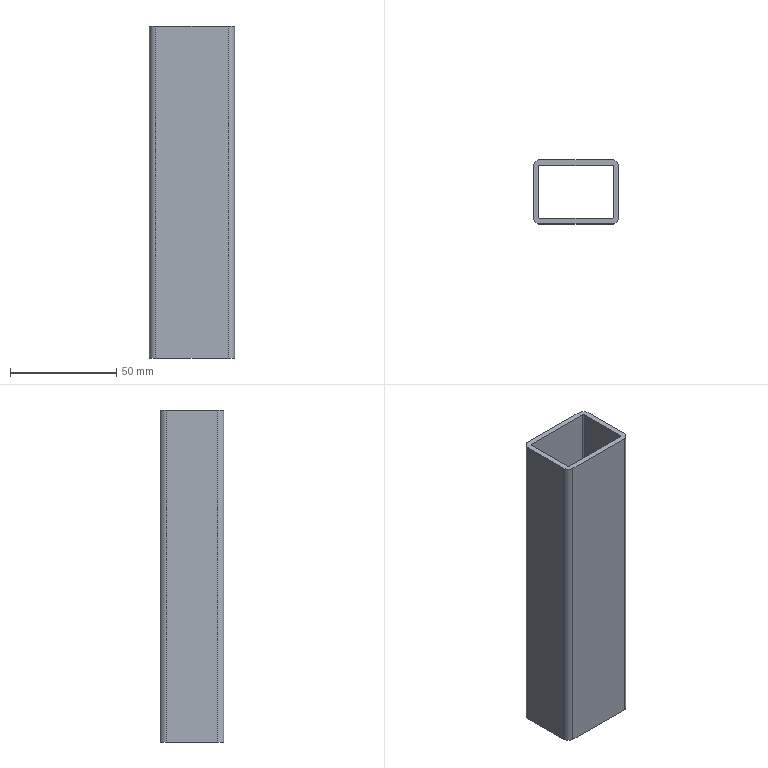Part | SolidWorks | features BaseBody 1 | 1 solid | 18 faces | box 40 x 30 x 156 mm | volume 49528 mm3 | plane 10 | cylinder 8 | commonest cylinder face diameters 1 x4 6 x4
STEP:
#1=CARTESIAN_POINT('',(17.,12.5,-78.));
#2=VERTEX_POINT('',#1);
#3=CARTESIAN_POINT('',(-17.,12.5,-78.));
#4=VERTEX_POINT('',#3);
#5=CARTESIAN_POINT('',(-17.,12.5,-78.));
#6=DIRECTION('',(-1.,0.,0.));
#7=VECTOR('',#6,1000.);
#8=LINE('',#5,#7);
#9=EDGE_CURVE('',#2,#4,#8,.T.);
#10=ORIENTED_EDGE('',*,*,#9,.F.);
#11=CARTESIAN_POINT('',(17.,12.5,78.));
#12=VERTEX_POINT('',#11);
#13=CARTESIAN_POINT('',(17.,12.5,78.));
#14=DIRECTION('',(0.,0.,-1.));
#15=VECTOR('',#14,1000.);
#16=LINE('',#13,#15);
#17=EDGE_CURVE('',#12,#2,#16,.T.);
#18=ORIENTED_EDGE('',*,*,#17,.F.);
#19=CARTESIAN_POINT('',(-17.,12.5,78.));
#20=VERTEX_POINT('',#19);
#21=CARTESIAN_POINT('',(-17.,12.5,78.));
#22=DIRECTION('',(-1.,0.,0.));
#23=VECTOR('',#22,1000.);
#24=LINE('',#21,#23);
#25=EDGE_CURVE('',#12,#20,#24,.T.);
#26=ORIENTED_EDGE('',*,*,#25,.T.);
#27=CARTESIAN_POINT('',(-17.,12.5,78.));
#28=DIRECTION('',(0.,0.,-1.));
#29=VECTOR('',#28,1000.);
#30=LINE('',#27,#29);
#31=EDGE_CURVE('',#20,#4,#30,.T.);
#32=ORIENTED_EDGE('',*,*,#31,.T.);
#33=EDGE_LOOP('',(#10,#18,#26,#32));
#34=FACE_OUTER_BOUND('',#33,.T.);
#35=CARTESIAN_POINT('',(-17.,12.5,78.));
#36=DIRECTION('',(0.,-1.,0.));
#37=DIRECTION('',(0.,0.,-1.));
#38=AXIS2_PLACEMENT_3D('',#35,#36,#37);
#39=PLANE('',#38);
#40=ADVANCED_FACE('',(#34),#39,.T.);
#41=CARTESIAN_POINT('',(17.5,12.,-78.));
#42=VERTEX_POINT('',#41);
#43=CARTESIAN_POINT('',(17.,12.,-78.));
#44=DIRECTION('',(0.,0.,1.));
#45=DIRECTION('',(-1.,0.,0.));
#46=AXIS2_PLACEMENT_3D('',#43,#44,#45);
#47=CIRCLE('',#46,0.5);
#48=EDGE_CURVE('',#42,#2,#47,.T.);
#49=ORIENTED_EDGE('',*,*,#48,.F.);
#50=CARTESIAN_POINT('',(17.5,12.,78.));
#51=VERTEX_POINT('',#50);
#52=CARTESIAN_POINT('',(17.5,12.,78.));
#53=DIRECTION('',(0.,0.,-1.));
#54=VECTOR('',#53,1000.);
#55=LINE('',#52,#54);
#56=EDGE_CURVE('',#51,#42,#55,.T.);
#57=ORIENTED_EDGE('',*,*,#56,.F.);
#58=CARTESIAN_POINT('',(17.,12.,78.));
#59=DIRECTION('',(0.,0.,1.));
#60=DIRECTION('',(-1.,0.,0.));
#61=AXIS2_PLACEMENT_3D('',#58,#59,#60);
#62=CIRCLE('',#61,0.5);
#63=EDGE_CURVE('',#51,#12,#62,.T.);
#64=ORIENTED_EDGE('',*,*,#63,.T.);
#65=ORIENTED_EDGE('',*,*,#17,.T.);
#66=EDGE_LOOP('',(#49,#57,#64,#65));
#67=FACE_OUTER_BOUND('',#66,.T.);
#68=CARTESIAN_POINT('',(17.,12.,78.));
#69=DIRECTION('',(0.,0.,-1.));
#70=DIRECTION('',(-1.,0.,0.));
#71=AXIS2_PLACEMENT_3D('',#68,#69,#70);
#72=CYLINDRICAL_SURFACE('',#71,0.5);
#73=ADVANCED_FACE('',(#67),#72,.F.);
#74=CARTESIAN_POINT('',(17.5,-12.,-78.));
#75=VERTEX_POINT('',#74);
#76=CARTESIAN_POINT('',(17.5,12.,-78.));
#77=DIRECTION('',(0.,1.,0.));
#78=VECTOR('',#77,1000.);
#79=LINE('',#76,#78);
#80=EDGE_CURVE('',#75,#42,#79,.T.);
#81=ORIENTED_EDGE('',*,*,#80,.F.);
#82=CARTESIAN_POINT('',(17.5,-12.,78.));
#83=VERTEX_POINT('',#82);
#84=CARTESIAN_POINT('',(17.5,-12.,78.));
#85=DIRECTION('',(0.,0.,-1.));
#86=VECTOR('',#85,1000.);
#87=LINE('',#84,#86);
#88=EDGE_CURVE('',#83,#75,#87,.T.);
#89=ORIENTED_EDGE('',*,*,#88,.F.);
#90=CARTESIAN_POINT('',(17.5,12.,78.));
#91=DIRECTION('',(0.,1.,0.));
#92=VECTOR('',#91,1000.);
#93=LINE('',#90,#92);
#94=EDGE_CURVE('',#83,#51,#93,.T.);
#95=ORIENTED_EDGE('',*,*,#94,.T.);
#96=ORIENTED_EDGE('',*,*,#56,.T.);
#97=EDGE_LOOP('',(#81,#89,#95,#96));
#98=FACE_OUTER_BOUND('',#97,.T.);
#99=CARTESIAN_POINT('',(17.5,12.,78.));
#100=DIRECTION('',(-1.,0.,0.));
#101=DIRECTION('',(0.,0.,1.));
#102=AXIS2_PLACEMENT_3D('',#99,#100,#101);
#103=PLANE('',#102);
#104=ADVANCED_FACE('',(#98),#103,.T.);
#105=CARTESIAN_POINT('',(17.,-12.5,-78.));
#106=VERTEX_POINT('',#105);
#107=CARTESIAN_POINT('',(17.,-12.,-78.));
#108=DIRECTION('',(0.,0.,1.));
#109=DIRECTION('',(1.,0.,0.));
#110=AXIS2_PLACEMENT_3D('',#107,#108,#109);
#111=CIRCLE('',#110,0.5);
#112=EDGE_CURVE('',#106,#75,#111,.T.);
#113=ORIENTED_EDGE('',*,*,#112,.F.);
#114=CARTESIAN_POINT('',(17.,-12.5,78.));
#115=VERTEX_POINT('',#114);
#116=CARTESIAN_POINT('',(17.,-12.5,78.));
#117=DIRECTION('',(0.,0.,-1.));
#118=VECTOR('',#117,1000.);
#119=LINE('',#116,#118);
#120=EDGE_CURVE('',#115,#106,#119,.T.);
#121=ORIENTED_EDGE('',*,*,#120,.F.);
#122=CARTESIAN_POINT('',(17.,-12.,78.));
#123=DIRECTION('',(0.,0.,1.));
#124=DIRECTION('',(1.,0.,0.));
#125=AXIS2_PLACEMENT_3D('',#122,#123,#124);
#126=CIRCLE('',#125,0.5);
#127=EDGE_CURVE('',#115,#83,#126,.T.);
#128=ORIENTED_EDGE('',*,*,#127,.T.);
#129=ORIENTED_EDGE('',*,*,#88,.T.);
#130=EDGE_LOOP('',(#113,#121,#128,#129));
#131=FACE_OUTER_BOUND('',#130,.T.);
#132=CARTESIAN_POINT('',(17.,-12.,78.));
#133=DIRECTION('',(0.,0.,-1.));
#134=DIRECTION('',(-1.,0.,0.));
#135=AXIS2_PLACEMENT_3D('',#132,#133,#134);
#136=CYLINDRICAL_SURFACE('',#135,0.5);
#137=ADVANCED_FACE('',(#131),#136,.F.);
#138=CARTESIAN_POINT('',(-17.,-12.5,-78.));
#139=VERTEX_POINT('',#138);
#140=CARTESIAN_POINT('',(-17.,-12.5,-78.));
#141=DIRECTION('',(1.,0.,0.));
#142=VECTOR('',#141,1000.);
#143=LINE('',#140,#142);
#144=EDGE_CURVE('',#139,#106,#143,.T.);
#145=ORIENTED_EDGE('',*,*,#144,.F.);
#146=CARTESIAN_POINT('',(-17.,-12.5,78.));
#147=VERTEX_POINT('',#146);
#148=CARTESIAN_POINT('',(-17.,-12.5,78.));
#149=DIRECTION('',(0.,0.,-1.));
#150=VECTOR('',#149,1000.);
#151=LINE('',#148,#150);
#152=EDGE_CURVE('',#147,#139,#151,.T.);
#153=ORIENTED_EDGE('',*,*,#152,.F.);
#154=CARTESIAN_POINT('',(-17.,-12.5,78.));
#155=DIRECTION('',(1.,0.,0.));
#156=VECTOR('',#155,1000.);
#157=LINE('',#154,#156);
#158=EDGE_CURVE('',#147,#115,#157,.T.);
#159=ORIENTED_EDGE('',*,*,#158,.T.);
#160=ORIENTED_EDGE('',*,*,#120,.T.);
#161=EDGE_LOOP('',(#145,#153,#159,#160));
#162=FACE_OUTER_BOUND('',#161,.T.);
#163=CARTESIAN_POINT('',(-17.,-12.5,78.));
#164=DIRECTION('',(0.,1.,0.));
#165=DIRECTION('',(1.,0.,0.));
#166=AXIS2_PLACEMENT_3D('',#163,#164,#165);
#167=PLANE('',#166);
#168=ADVANCED_FACE('',(#162),#167,.T.);
#169=CARTESIAN_POINT('',(-17.5,-12.,-78.));
#170=VERTEX_POINT('',#169);
#171=CARTESIAN_POINT('',(-17.,-12.,-78.));
#172=DIRECTION('',(0.,0.,1.));
#173=DIRECTION('',(1.,0.,0.));
#174=AXIS2_PLACEMENT_3D('',#171,#172,#173);
#175=CIRCLE('',#174,0.5);
#176=EDGE_CURVE('',#170,#139,#175,.T.);
#177=ORIENTED_EDGE('',*,*,#176,.F.);
#178=CARTESIAN_POINT('',(-17.5,-12.,78.));
#179=VERTEX_POINT('',#178);
#180=CARTESIAN_POINT('',(-17.5,-12.,78.));
#181=DIRECTION('',(0.,0.,-1.));
#182=VECTOR('',#181,1000.);
#183=LINE('',#180,#182);
#184=EDGE_CURVE('',#179,#170,#183,.T.);
#185=ORIENTED_EDGE('',*,*,#184,.F.);
#186=CARTESIAN_POINT('',(-17.,-12.,78.));
#187=DIRECTION('',(0.,0.,1.));
#188=DIRECTION('',(1.,0.,0.));
#189=AXIS2_PLACEMENT_3D('',#186,#187,#188);
#190=CIRCLE('',#189,0.5);
#191=EDGE_CURVE('',#179,#147,#190,.T.);
#192=ORIENTED_EDGE('',*,*,#191,.T.);
#193=ORIENTED_EDGE('',*,*,#152,.T.);
#194=EDGE_LOOP('',(#177,#185,#192,#193));
#195=FACE_OUTER_BOUND('',#194,.T.);
#196=CARTESIAN_POINT('',(-17.,-12.,78.));
#197=DIRECTION('',(0.,0.,-1.));
#198=DIRECTION('',(-1.,0.,0.));
#199=AXIS2_PLACEMENT_3D('',#196,#197,#198);
#200=CYLINDRICAL_SURFACE('',#199,0.5);
#201=ADVANCED_FACE('',(#195),#200,.F.);
#202=CARTESIAN_POINT('',(-17.5,12.,-78.));
#203=VERTEX_POINT('',#202);
#204=CARTESIAN_POINT('',(-17.5,12.,-78.));
#205=DIRECTION('',(0.,-1.,0.));
#206=VECTOR('',#205,1000.);
#207=LINE('',#204,#206);
#208=EDGE_CURVE('',#203,#170,#207,.T.);
#209=ORIENTED_EDGE('',*,*,#208,.F.);
#210=CARTESIAN_POINT('',(-17.5,12.,78.));
#211=VERTEX_POINT('',#210);
#212=CARTESIAN_POINT('',(-17.5,12.,78.));
#213=DIRECTION('',(0.,0.,-1.));
#214=VECTOR('',#213,1000.);
#215=LINE('',#212,#214);
#216=EDGE_CURVE('',#211,#203,#215,.T.);
#217=ORIENTED_EDGE('',*,*,#216,.F.);
#218=CARTESIAN_POINT('',(-17.5,12.,78.));
#219=DIRECTION('',(0.,-1.,0.));
#220=VECTOR('',#219,1000.);
#221=LINE('',#218,#220);
#222=EDGE_CURVE('',#211,#179,#221,.T.);
#223=ORIENTED_EDGE('',*,*,#222,.T.);
#224=ORIENTED_EDGE('',*,*,#184,.T.);
#225=EDGE_LOOP('',(#209,#217,#223,#224));
#226=FACE_OUTER_BOUND('',#225,.T.);
#227=CARTESIAN_POINT('',(-17.5,12.,78.));
#228=DIRECTION('',(1.,0.,0.));
#229=DIRECTION('',(0.,1.,0.));
#230=AXIS2_PLACEMENT_3D('',#227,#228,#229);
#231=PLANE('',#230);
#232=ADVANCED_FACE('',(#226),#231,.T.);
#233=CARTESIAN_POINT('',(-17.,12.,-78.));
#234=DIRECTION('',(0.,0.,1.));
#235=DIRECTION('',(1.,0.,0.));
#236=AXIS2_PLACEMENT_3D('',#233,#234,#235);
#237=CIRCLE('',#236,0.5);
#238=EDGE_CURVE('',#4,#203,#237,.T.);
#239=ORIENTED_EDGE('',*,*,#238,.F.);
#240=ORIENTED_EDGE('',*,*,#31,.F.);
#241=CARTESIAN_POINT('',(-17.,12.,78.));
#242=DIRECTION('',(0.,0.,1.));
#243=DIRECTION('',(1.,0.,0.));
#244=AXIS2_PLACEMENT_3D('',#241,#242,#243);
#245=CIRCLE('',#244,0.5);
#246=EDGE_CURVE('',#20,#211,#245,.T.);
#247=ORIENTED_EDGE('',*,*,#246,.T.);
#248=ORIENTED_EDGE('',*,*,#216,.T.);
#249=EDGE_LOOP('',(#239,#240,#247,#248));
#250=FACE_OUTER_BOUND('',#249,.T.);
#251=CARTESIAN_POINT('',(-17.,12.,78.));
#252=DIRECTION('',(0.,0.,-1.));
#253=DIRECTION('',(-1.,0.,0.));
#254=AXIS2_PLACEMENT_3D('',#251,#252,#253);
#255=CYLINDRICAL_SURFACE('',#254,0.5);
#256=ADVANCED_FACE('',(#250),#255,.F.);
#257=CARTESIAN_POINT('',(-20.,12.,-78.));
#258=VERTEX_POINT('',#257);
#259=CARTESIAN_POINT('',(-20.,-12.,-78.));
#260=VERTEX_POINT('',#259);
#261=CARTESIAN_POINT('',(-20.,12.,-78.));
#262=DIRECTION('',(0.,-1.,0.));
#263=VECTOR('',#262,1000.);
#264=LINE('',#261,#263);
#265=EDGE_CURVE('',#258,#260,#264,.T.);
#266=ORIENTED_EDGE('',*,*,#265,.T.);
#267=CARTESIAN_POINT('',(-20.,-12.,78.));
#268=VERTEX_POINT('',#267);
#269=CARTESIAN_POINT('',(-20.,-12.,78.));
#270=DIRECTION('',(0.,0.,-1.));
#271=VECTOR('',#270,1000.);
#272=LINE('',#269,#271);
#273=EDGE_CURVE('',#268,#260,#272,.T.);
#274=ORIENTED_EDGE('',*,*,#273,.F.);
#275=CARTESIAN_POINT('',(-20.,12.,78.));
#276=VERTEX_POINT('',#275);
#277=CARTESIAN_POINT('',(-20.,12.,78.));
#278=DIRECTION('',(0.,-1.,0.));
#279=VECTOR('',#278,1000.);
#280=LINE('',#277,#279);
#281=EDGE_CURVE('',#276,#268,#280,.T.);
#282=ORIENTED_EDGE('',*,*,#281,.F.);
#283=CARTESIAN_POINT('',(-20.,12.,78.));
#284=DIRECTION('',(0.,0.,-1.));
#285=VECTOR('',#284,1000.);
#286=LINE('',#283,#285);
#287=EDGE_CURVE('',#276,#258,#286,.T.);
#288=ORIENTED_EDGE('',*,*,#287,.T.);
#289=EDGE_LOOP('',(#266,#274,#282,#288));
#290=FACE_OUTER_BOUND('',#289,.T.);
#291=CARTESIAN_POINT('',(-20.,12.,78.));
#292=DIRECTION('',(1.,0.,0.));
#293=DIRECTION('',(0.,1.,0.));
#294=AXIS2_PLACEMENT_3D('',#291,#292,#293);
#295=PLANE('',#294);
#296=ADVANCED_FACE('',(#290),#295,.F.);
#297=CARTESIAN_POINT('',(-17.,15.,-78.));
#298=VERTEX_POINT('',#297);
#299=CARTESIAN_POINT('',(-17.,12.,-78.));
#300=DIRECTION('',(0.,0.,1.));
#301=DIRECTION('',(1.,0.,0.));
#302=AXIS2_PLACEMENT_3D('',#299,#300,#301);
#303=CIRCLE('',#302,3.);
#304=EDGE_CURVE('',#298,#258,#303,.T.);
#305=ORIENTED_EDGE('',*,*,#304,.T.);
#306=ORIENTED_EDGE('',*,*,#287,.F.);
#307=CARTESIAN_POINT('',(-17.,15.,78.));
#308=VERTEX_POINT('',#307);
#309=CARTESIAN_POINT('',(-17.,12.,78.));
#310=DIRECTION('',(0.,0.,1.));
#311=DIRECTION('',(1.,0.,0.));
#312=AXIS2_PLACEMENT_3D('',#309,#310,#311);
#313=CIRCLE('',#312,3.);
#314=EDGE_CURVE('',#308,#276,#313,.T.);
#315=ORIENTED_EDGE('',*,*,#314,.F.);
#316=CARTESIAN_POINT('',(-17.,15.,78.));
#317=DIRECTION('',(0.,0.,-1.));
#318=VECTOR('',#317,1000.);
#319=LINE('',#316,#318);
#320=EDGE_CURVE('',#308,#298,#319,.T.);
#321=ORIENTED_EDGE('',*,*,#320,.T.);
#322=EDGE_LOOP('',(#305,#306,#315,#321));
#323=FACE_OUTER_BOUND('',#322,.T.);
#324=CARTESIAN_POINT('',(-17.,12.,78.));
#325=DIRECTION('',(0.,0.,-1.));
#326=DIRECTION('',(-1.,0.,0.));
#327=AXIS2_PLACEMENT_3D('',#324,#325,#326);
#328=CYLINDRICAL_SURFACE('',#327,3.);
#329=ADVANCED_FACE('',(#323),#328,.T.);
#330=CARTESIAN_POINT('',(17.,15.,-78.));
#331=VERTEX_POINT('',#330);
#332=CARTESIAN_POINT('',(-17.,15.,-78.));
#333=DIRECTION('',(-1.,0.,0.));
#334=VECTOR('',#333,1000.);
#335=LINE('',#332,#334);
#336=EDGE_CURVE('',#331,#298,#335,.T.);
#337=ORIENTED_EDGE('',*,*,#336,.T.);
#338=ORIENTED_EDGE('',*,*,#320,.F.);
#339=CARTESIAN_POINT('',(17.,15.,78.));
#340=VERTEX_POINT('',#339);
#341=CARTESIAN_POINT('',(-17.,15.,78.));
#342=DIRECTION('',(-1.,0.,0.));
#343=VECTOR('',#342,1000.);
#344=LINE('',#341,#343);
#345=EDGE_CURVE('',#340,#308,#344,.T.);
#346=ORIENTED_EDGE('',*,*,#345,.F.);
#347=CARTESIAN_POINT('',(17.,15.,78.));
#348=DIRECTION('',(0.,0.,-1.));
#349=VECTOR('',#348,1000.);
#350=LINE('',#347,#349);
#351=EDGE_CURVE('',#340,#331,#350,.T.);
#352=ORIENTED_EDGE('',*,*,#351,.T.);
#353=EDGE_LOOP('',(#337,#338,#346,#352));
#354=FACE_OUTER_BOUND('',#353,.T.);
#355=CARTESIAN_POINT('',(-17.,15.,78.));
#356=DIRECTION('',(0.,-1.,0.));
#357=DIRECTION('',(0.,0.,-1.));
#358=AXIS2_PLACEMENT_3D('',#355,#356,#357);
#359=PLANE('',#358);
#360=ADVANCED_FACE('',(#354),#359,.F.);
#361=CARTESIAN_POINT('',(20.,12.,-78.));
#362=VERTEX_POINT('',#361);
#363=CARTESIAN_POINT('',(17.,12.,-78.));
#364=DIRECTION('',(0.,0.,1.));
#365=DIRECTION('',(-1.,0.,0.));
#366=AXIS2_PLACEMENT_3D('',#363,#364,#365);
#367=CIRCLE('',#366,3.);
#368=EDGE_CURVE('',#362,#331,#367,.T.);
#369=ORIENTED_EDGE('',*,*,#368,.T.);
#370=ORIENTED_EDGE('',*,*,#351,.F.);
#371=CARTESIAN_POINT('',(20.,12.,78.));
#372=VERTEX_POINT('',#371);
#373=CARTESIAN_POINT('',(17.,12.,78.));
#374=DIRECTION('',(0.,0.,1.));
#375=DIRECTION('',(-1.,0.,0.));
#376=AXIS2_PLACEMENT_3D('',#373,#374,#375);
#377=CIRCLE('',#376,3.);
#378=EDGE_CURVE('',#372,#340,#377,.T.);
#379=ORIENTED_EDGE('',*,*,#378,.F.);
#380=CARTESIAN_POINT('',(20.,12.,78.));
#381=DIRECTION('',(0.,0.,-1.));
#382=VECTOR('',#381,1000.);
#383=LINE('',#380,#382);
#384=EDGE_CURVE('',#372,#362,#383,.T.);
#385=ORIENTED_EDGE('',*,*,#384,.T.);
#386=EDGE_LOOP('',(#369,#370,#379,#385));
#387=FACE_OUTER_BOUND('',#386,.T.);
#388=CARTESIAN_POINT('',(17.,12.,78.));
#389=DIRECTION('',(0.,0.,-1.));
#390=DIRECTION('',(-1.,0.,0.));
#391=AXIS2_PLACEMENT_3D('',#388,#389,#390);
#392=CYLINDRICAL_SURFACE('',#391,3.);
#393=ADVANCED_FACE('',(#387),#392,.T.);
#394=CARTESIAN_POINT('',(20.,-12.,-78.));
#395=VERTEX_POINT('',#394);
#396=CARTESIAN_POINT('',(20.,12.,-78.));
#397=DIRECTION('',(0.,1.,0.));
#398=VECTOR('',#397,1000.);
#399=LINE('',#396,#398);
#400=EDGE_CURVE('',#395,#362,#399,.T.);
#401=ORIENTED_EDGE('',*,*,#400,.T.);
#402=ORIENTED_EDGE('',*,*,#384,.F.);
#403=CARTESIAN_POINT('',(20.,-12.,78.));
#404=VERTEX_POINT('',#403);
#405=CARTESIAN_POINT('',(20.,12.,78.));
#406=DIRECTION('',(0.,1.,0.));
#407=VECTOR('',#406,1000.);
#408=LINE('',#405,#407);
#409=EDGE_CURVE('',#404,#372,#408,.T.);
#410=ORIENTED_EDGE('',*,*,#409,.F.);
#411=CARTESIAN_POINT('',(20.,-12.,78.));
#412=DIRECTION('',(0.,0.,-1.));
#413=VECTOR('',#412,1000.);
#414=LINE('',#411,#413);
#415=EDGE_CURVE('',#404,#395,#414,.T.);
#416=ORIENTED_EDGE('',*,*,#415,.T.);
#417=EDGE_LOOP('',(#401,#402,#410,#416));
#418=FACE_OUTER_BOUND('',#417,.T.);
#419=CARTESIAN_POINT('',(20.,12.,78.));
#420=DIRECTION('',(-1.,0.,0.));
#421=DIRECTION('',(0.,1.,0.));
#422=AXIS2_PLACEMENT_3D('',#419,#420,#421);
#423=PLANE('',#422);
#424=ADVANCED_FACE('',(#418),#423,.F.);
#425=CARTESIAN_POINT('',(17.,-15.,-78.));
#426=VERTEX_POINT('',#425);
#427=CARTESIAN_POINT('',(17.,-12.,-78.));
#428=DIRECTION('',(0.,0.,1.));
#429=DIRECTION('',(1.,0.,0.));
#430=AXIS2_PLACEMENT_3D('',#427,#428,#429);
#431=CIRCLE('',#430,3.);
#432=EDGE_CURVE('',#426,#395,#431,.T.);
#433=ORIENTED_EDGE('',*,*,#432,.T.);
#434=ORIENTED_EDGE('',*,*,#415,.F.);
#435=CARTESIAN_POINT('',(17.,-15.,78.));
#436=VERTEX_POINT('',#435);
#437=CARTESIAN_POINT('',(17.,-12.,78.));
#438=DIRECTION('',(0.,0.,1.));
#439=DIRECTION('',(1.,0.,0.));
#440=AXIS2_PLACEMENT_3D('',#437,#438,#439);
#441=CIRCLE('',#440,3.);
#442=EDGE_CURVE('',#436,#404,#441,.T.);
#443=ORIENTED_EDGE('',*,*,#442,.F.);
#444=CARTESIAN_POINT('',(17.,-15.,78.));
#445=DIRECTION('',(0.,0.,-1.));
#446=VECTOR('',#445,1000.);
#447=LINE('',#444,#446);
#448=EDGE_CURVE('',#436,#426,#447,.T.);
#449=ORIENTED_EDGE('',*,*,#448,.T.);
#450=EDGE_LOOP('',(#433,#434,#443,#449));
#451=FACE_OUTER_BOUND('',#450,.T.);
#452=CARTESIAN_POINT('',(17.,-12.,78.));
#453=DIRECTION('',(0.,0.,-1.));
#454=DIRECTION('',(-1.,0.,0.));
#455=AXIS2_PLACEMENT_3D('',#452,#453,#454);
#456=CYLINDRICAL_SURFACE('',#455,3.);
#457=ADVANCED_FACE('',(#451),#456,.T.);
#458=CARTESIAN_POINT('',(-17.,-15.,-78.));
#459=VERTEX_POINT('',#458);
#460=CARTESIAN_POINT('',(-17.,-15.,-78.));
#461=DIRECTION('',(1.,0.,0.));
#462=VECTOR('',#461,1000.);
#463=LINE('',#460,#462);
#464=EDGE_CURVE('',#459,#426,#463,.T.);
#465=ORIENTED_EDGE('',*,*,#464,.T.);
#466=ORIENTED_EDGE('',*,*,#448,.F.);
#467=CARTESIAN_POINT('',(-17.,-15.,78.));
#468=VERTEX_POINT('',#467);
#469=CARTESIAN_POINT('',(-17.,-15.,78.));
#470=DIRECTION('',(1.,0.,0.));
#471=VECTOR('',#470,1000.);
#472=LINE('',#469,#471);
#473=EDGE_CURVE('',#468,#436,#472,.T.);
#474=ORIENTED_EDGE('',*,*,#473,.F.);
#475=CARTESIAN_POINT('',(-17.,-15.,78.));
#476=DIRECTION('',(0.,0.,-1.));
#477=VECTOR('',#476,1000.);
#478=LINE('',#475,#477);
#479=EDGE_CURVE('',#468,#459,#478,.T.);
#480=ORIENTED_EDGE('',*,*,#479,.T.);
#481=EDGE_LOOP('',(#465,#466,#474,#480));
#482=FACE_OUTER_BOUND('',#481,.T.);
#483=CARTESIAN_POINT('',(-17.,-15.,78.));
#484=DIRECTION('',(0.,1.,0.));
#485=DIRECTION('',(1.,0.,0.));
#486=AXIS2_PLACEMENT_3D('',#483,#484,#485);
#487=PLANE('',#486);
#488=ADVANCED_FACE('',(#482),#487,.F.);
#489=CARTESIAN_POINT('',(-17.,-12.,-78.));
#490=DIRECTION('',(0.,0.,1.));
#491=DIRECTION('',(1.,0.,0.));
#492=AXIS2_PLACEMENT_3D('',#489,#490,#491);
#493=CIRCLE('',#492,3.);
#494=EDGE_CURVE('',#260,#459,#493,.T.);
#495=ORIENTED_EDGE('',*,*,#494,.T.);
#496=ORIENTED_EDGE('',*,*,#479,.F.);
#497=CARTESIAN_POINT('',(-17.,-12.,78.));
#498=DIRECTION('',(0.,0.,1.));
#499=DIRECTION('',(1.,0.,0.));
#500=AXIS2_PLACEMENT_3D('',#497,#498,#499);
#501=CIRCLE('',#500,3.);
#502=EDGE_CURVE('',#268,#468,#501,.T.);
#503=ORIENTED_EDGE('',*,*,#502,.F.);
#504=ORIENTED_EDGE('',*,*,#273,.T.);
#505=EDGE_LOOP('',(#495,#496,#503,#504));
#506=FACE_OUTER_BOUND('',#505,.T.);
#507=CARTESIAN_POINT('',(-17.,-12.,78.));
#508=DIRECTION('',(0.,0.,-1.));
#509=DIRECTION('',(-1.,0.,0.));
#510=AXIS2_PLACEMENT_3D('',#507,#508,#509);
#511=CYLINDRICAL_SURFACE('',#510,3.);
#512=ADVANCED_FACE('',(#506),#511,.T.);
#513=ORIENTED_EDGE('',*,*,#238,.T.);
#514=ORIENTED_EDGE('',*,*,#208,.T.);
#515=ORIENTED_EDGE('',*,*,#176,.T.);
#516=ORIENTED_EDGE('',*,*,#144,.T.);
#517=ORIENTED_EDGE('',*,*,#112,.T.);
#518=ORIENTED_EDGE('',*,*,#80,.T.);
#519=ORIENTED_EDGE('',*,*,#48,.T.);
#520=ORIENTED_EDGE('',*,*,#9,.T.);
#521=EDGE_LOOP('',(#513,#514,#515,#516,#517,#518,#519,#520));
#522=FACE_BOUND('',#521,.T.);
#523=ORIENTED_EDGE('',*,*,#494,.F.);
#524=ORIENTED_EDGE('',*,*,#265,.F.);
#525=ORIENTED_EDGE('',*,*,#304,.F.);
#526=ORIENTED_EDGE('',*,*,#336,.F.);
#527=ORIENTED_EDGE('',*,*,#368,.F.);
#528=ORIENTED_EDGE('',*,*,#400,.F.);
#529=ORIENTED_EDGE('',*,*,#432,.F.);
#530=ORIENTED_EDGE('',*,*,#464,.F.);
#531=EDGE_LOOP('',(#523,#524,#525,#526,#527,#528,#529,#530));
#532=FACE_OUTER_BOUND('',#531,.T.);
#533=CARTESIAN_POINT('',(-17.,-12.,-78.));
#534=DIRECTION('',(0.,0.,1.));
#535=DIRECTION('',(1.,0.,0.));
#536=AXIS2_PLACEMENT_3D('',#533,#534,#535);
#537=PLANE('',#536);
#538=ADVANCED_FACE('',(#522,#532),#537,.F.);
#539=ORIENTED_EDGE('',*,*,#222,.F.);
#540=ORIENTED_EDGE('',*,*,#246,.F.);
#541=ORIENTED_EDGE('',*,*,#25,.F.);
#542=ORIENTED_EDGE('',*,*,#63,.F.);
#543=ORIENTED_EDGE('',*,*,#94,.F.);
#544=ORIENTED_EDGE('',*,*,#127,.F.);
#545=ORIENTED_EDGE('',*,*,#158,.F.);
#546=ORIENTED_EDGE('',*,*,#191,.F.);
#547=EDGE_LOOP('',(#539,#540,#541,#542,#543,#544,#545,#546));
#548=FACE_BOUND('',#547,.T.);
#549=ORIENTED_EDGE('',*,*,#502,.T.);
#550=ORIENTED_EDGE('',*,*,#473,.T.);
#551=ORIENTED_EDGE('',*,*,#442,.T.);
#552=ORIENTED_EDGE('',*,*,#409,.T.);
#553=ORIENTED_EDGE('',*,*,#378,.T.);
#554=ORIENTED_EDGE('',*,*,#345,.T.);
#555=ORIENTED_EDGE('',*,*,#314,.T.);
#556=ORIENTED_EDGE('',*,*,#281,.T.);
#557=EDGE_LOOP('',(#549,#550,#551,#552,#553,#554,#555,#556));
#558=FACE_OUTER_BOUND('',#557,.T.);
#559=CARTESIAN_POINT('',(-17.,-12.,78.));
#560=DIRECTION('',(0.,0.,1.));
#561=DIRECTION('',(1.,0.,0.));
#562=AXIS2_PLACEMENT_3D('',#559,#560,#561);
#563=PLANE('',#562);
#564=ADVANCED_FACE('',(#548,#558),#563,.T.);
#565=CLOSED_SHELL('',(#40,#73,#104,#137,#168,#201,#232,#256,#296,#329,#360,#393,#424,#457,#488,#512,#538,#564));
#566=MANIFOLD_SOLID_BREP('',#565);
#567=CARTESIAN_POINT('',(0.,0.,0.));
#568=DIRECTION('',(0.,0.,1.));
#569=DIRECTION('',(1.,0.,0.));
#570=AXIS2_PLACEMENT_3D('',#567,#568,#569);
#571=(LENGTH_UNIT()NAMED_UNIT(*)SI_UNIT(.MILLI.,.METRE.));
#572=UNCERTAINTY_MEASURE_WITH_UNIT(LENGTH_MEASURE(0.00001),#571,'','');
#573=(NAMED_UNIT(*)PLANE_ANGLE_UNIT()SI_UNIT($,.RADIAN.));
#574=(NAMED_UNIT(*)SI_UNIT($,.STERADIAN.)SOLID_ANGLE_UNIT());
#575=(GEOMETRIC_REPRESENTATION_CONTEXT(3)GLOBAL_UNCERTAINTY_ASSIGNED_CONTEXT((#572))GLOBAL_UNIT_ASSIGNED_CONTEXT((#571,#573,#574))REPRESENTATION_CONTEXT('',''));
#576=ADVANCED_BREP_SHAPE_REPRESENTATION('',(#566,#570),#575);